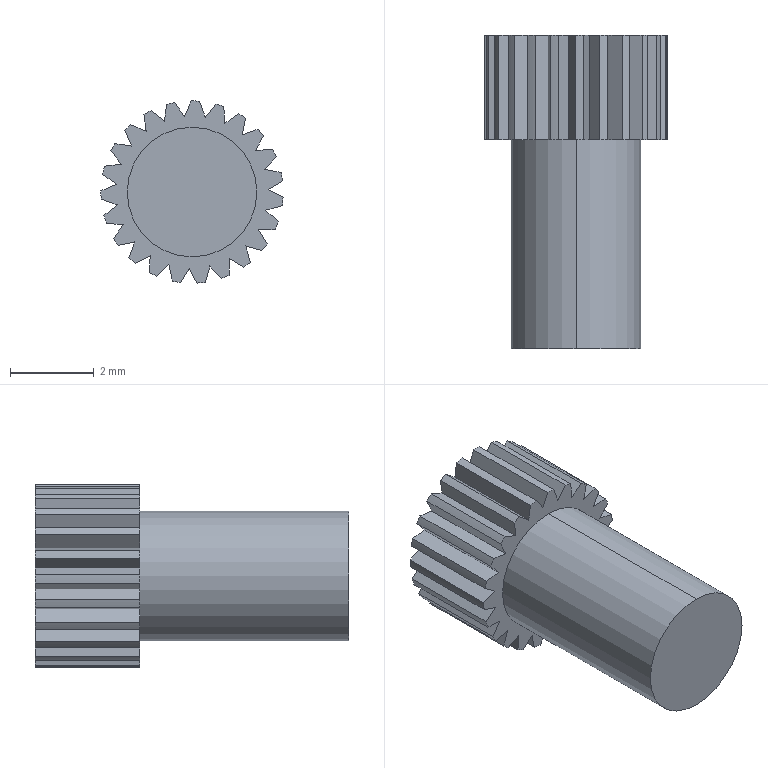Part | SolidWorks | features CombineBodies 2, MoveCopyBody 2, Stock 2, Extrusion 1, ICE 1 | 1 solid | 103 faces | box 4.357 x 7.5 x 4.358 mm | volume 48.395 mm3 | plane 51 | cylinder 43 | spline 9 | commonest cylinder face diameters 4.361 x23 2.86 x18 3.1 x2